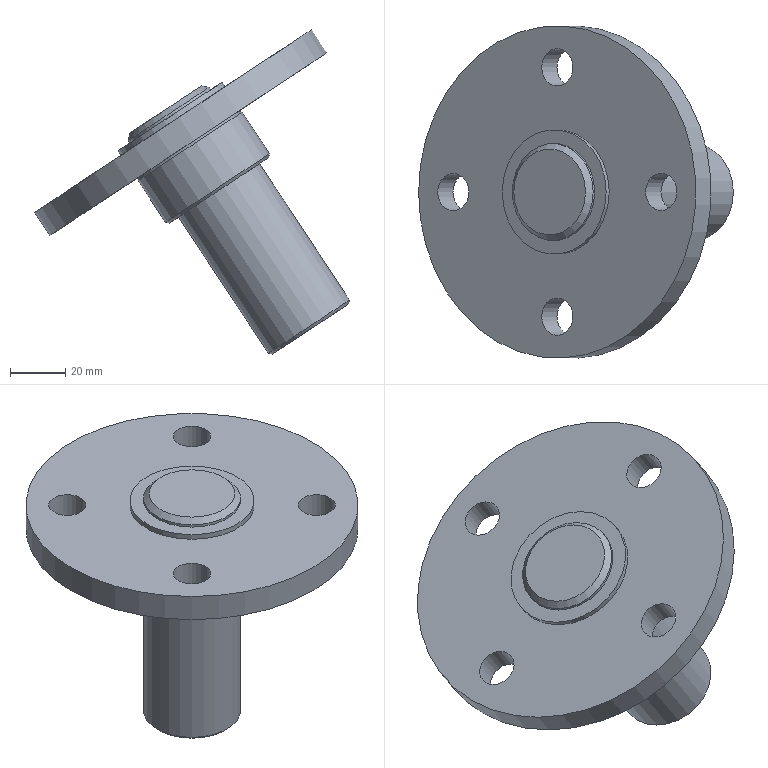Part | STEP file | HL4GZ-1.862.034 (flange rotating shaft) | 2 solids | 21 faces | box 113.701 x 120 x 117.252 mm | volume 202570 mm3 | cylinder 10 | plane 7 | cone 4 | commonest cylinder face diameters 13.5 x4 35 x3 45 x2 120 x1
STEP:
#1=CARTESIAN_POINT('',(0.,0.,0.));
#2=DIRECTION('',(0.,0.,1.));
#3=DIRECTION('',(1.,0.,0.));
#4=AXIS2_PLACEMENT_3D('',#1,#2,#3);
#5=CARTESIAN_POINT('',(3828.992,-590.,-108.754));
#6=VERTEX_POINT('',#5);
#7=CARTESIAN_POINT('',(3843.599,-590.,-99.117));
#8=DIRECTION('',(0.5507,0.,-0.8347));
#9=DIRECTION('',(-0.8347,0.,-0.5507));
#10=AXIS2_PLACEMENT_3D('',#7,#8,#9);
#11=CIRCLE('',#10,17.5);
#12=CARTESIAN_POINT('',(3843.599,-590.,-99.117));
#13=DIRECTION('',(0.5507,0.,-0.8347));
#14=DIRECTION('',(-0.8347,0.,-0.5507));
#15=AXIS2_PLACEMENT_3D('',#12,#13,#14);
#16=PLANE('',#15);
#17=CARTESIAN_POINT('',(0.,0.));
#18=DIRECTION('',(1.,0.));
#19=AXIS2_PLACEMENT_2D('',#17,#18);
#20=CIRCLE('',#19,17.5);
#21=(GEOMETRIC_REPRESENTATION_CONTEXT(2)PARAMETRIC_REPRESENTATION_CONTEXT()REPRESENTATION_CONTEXT('',''));
#22=DEFINITIONAL_REPRESENTATION('',(#20),#21);
#23=PCURVE('',#16,#22);
#24=CARTESIAN_POINT('',(3846.903,-590.,-104.125));
#25=DIRECTION('',(0.5507,0.,-0.8347));
#26=DIRECTION('',(0.8347,0.,0.5507));
#27=AXIS2_PLACEMENT_3D('',#24,#25,#26);
#28=CYLINDRICAL_SURFACE('',#27,17.5);
#29=CARTESIAN_POINT('',(3.142,-6.));
#30=DIRECTION('',(1.,0.));
#31=VECTOR('',#30,1.);
#32=LINE('',#29,#31);
#33=(GEOMETRIC_REPRESENTATION_CONTEXT(2)PARAMETRIC_REPRESENTATION_CONTEXT()REPRESENTATION_CONTEXT('',''));
#34=DEFINITIONAL_REPRESENTATION('',(#32),#33);
#35=PCURVE('',#28,#34);
#36=SURFACE_CURVE('',#11,(#23,#35),.PCURVE_S1.);
#37=EDGE_CURVE('',#6,#6,#36,.T.);
#38=ORIENTED_EDGE('',*,*,#37,.T.);
#39=EDGE_LOOP('',(#38));
#40=FACE_BOUND('',#39,.T.);
#41=CARTESIAN_POINT('',(3824.818,-590.,-111.507));
#42=VERTEX_POINT('',#41);
#43=CARTESIAN_POINT('',(3843.599,-590.,-99.117));
#44=DIRECTION('',(-0.5507,0.,0.8347));
#45=DIRECTION('',(-0.8347,0.,-0.5507));
#46=AXIS2_PLACEMENT_3D('',#43,#44,#45);
#47=CIRCLE('',#46,22.5);
#48=CARTESIAN_POINT('',(22.5,0.));
#49=CARTESIAN_POINT('',(22.5,-38.971));
#50=CARTESIAN_POINT('',(-11.25,-19.486));
#51=CARTESIAN_POINT('',(-45.,0.));
#52=CARTESIAN_POINT('',(-11.25,19.486));
#53=CARTESIAN_POINT('',(22.5,38.971));
#54=CARTESIAN_POINT('',(22.5,0.));
#55=(BOUNDED_CURVE()B_SPLINE_CURVE(2,(#48,#49,#50,#51,#52,#53,#54),.UNSPECIFIED.,.T.,.F.)B_SPLINE_CURVE_WITH_KNOTS((1,2,2,2,2,1),(-2.094,0.,2.094,4.189,6.283,8.378),.UNSPECIFIED.)CURVE()GEOMETRIC_REPRESENTATION_ITEM()RATIONAL_B_SPLINE_CURVE((1.,0.5,1.,0.5,1.,0.5,1.))REPRESENTATION_ITEM(''));
#56=(GEOMETRIC_REPRESENTATION_CONTEXT(2)PARAMETRIC_REPRESENTATION_CONTEXT()REPRESENTATION_CONTEXT('',''));
#57=DEFINITIONAL_REPRESENTATION('',(#55),#56);
#58=PCURVE('',#16,#57);
#59=CARTESIAN_POINT('',(3844.7,-590.,-100.786));
#60=DIRECTION('',(0.5507,0.,-0.8347));
#61=DIRECTION('',(0.8347,0.,0.5507));
#62=AXIS2_PLACEMENT_3D('',#59,#60,#61);
#63=CYLINDRICAL_SURFACE('',#62,22.5);
#64=CARTESIAN_POINT('',(9.425,-2.));
#65=DIRECTION('',(-1.,0.));
#66=VECTOR('',#65,1.);
#67=LINE('',#64,#66);
#68=(GEOMETRIC_REPRESENTATION_CONTEXT(2)PARAMETRIC_REPRESENTATION_CONTEXT()REPRESENTATION_CONTEXT('',''));
#69=DEFINITIONAL_REPRESENTATION('',(#67),#68);
#70=PCURVE('',#63,#69);
#71=SURFACE_CURVE('',#47,(#58,#70),.PCURVE_S1.);
#72=EDGE_CURVE('',#42,#42,#71,.T.);
#73=ORIENTED_EDGE('',*,*,#72,.T.);
#74=EDGE_LOOP('',(#73));
#75=FACE_BOUND('',#74,.T.);
#76=ADVANCED_FACE('',(#40,#75),#16,.F.);
#77=CARTESIAN_POINT('',(3825.919,-590.,-113.176));
#78=VERTEX_POINT('',#77);
#79=CARTESIAN_POINT('',(3844.7,-590.,-100.786));
#80=DIRECTION('',(-0.5507,0.,0.8347));
#81=DIRECTION('',(-0.8347,0.,-0.5507));
#82=AXIS2_PLACEMENT_3D('',#79,#80,#81);
#83=CIRCLE('',#82,22.5);
#84=CARTESIAN_POINT('',(9.425,0.));
#85=DIRECTION('',(-1.,0.));
#86=VECTOR('',#85,1.);
#87=LINE('',#84,#86);
#88=(GEOMETRIC_REPRESENTATION_CONTEXT(2)PARAMETRIC_REPRESENTATION_CONTEXT()REPRESENTATION_CONTEXT('',''));
#89=DEFINITIONAL_REPRESENTATION('',(#87),#88);
#90=PCURVE('',#63,#89);
#91=CARTESIAN_POINT('',(3844.7,-590.,-100.786));
#92=DIRECTION('',(0.5507,0.,-0.8347));
#93=DIRECTION('',(-0.8347,0.,-0.5507));
#94=AXIS2_PLACEMENT_3D('',#91,#92,#93);
#95=PLANE('',#94);
#96=CARTESIAN_POINT('',(22.5,0.));
#97=CARTESIAN_POINT('',(22.5,-38.971));
#98=CARTESIAN_POINT('',(-11.25,-19.486));
#99=CARTESIAN_POINT('',(-45.,0.));
#100=CARTESIAN_POINT('',(-11.25,19.486));
#101=CARTESIAN_POINT('',(22.5,38.971));
#102=CARTESIAN_POINT('',(22.5,0.));
#103=(BOUNDED_CURVE()B_SPLINE_CURVE(2,(#96,#97,#98,#99,#100,#101,#102),.UNSPECIFIED.,.T.,.F.)B_SPLINE_CURVE_WITH_KNOTS((1,2,2,2,2,1),(-2.094,0.,2.094,4.189,6.283,8.378),.UNSPECIFIED.)CURVE()GEOMETRIC_REPRESENTATION_ITEM()RATIONAL_B_SPLINE_CURVE((1.,0.5,1.,0.5,1.,0.5,1.))REPRESENTATION_ITEM(''));
#104=(GEOMETRIC_REPRESENTATION_CONTEXT(2)PARAMETRIC_REPRESENTATION_CONTEXT()REPRESENTATION_CONTEXT('',''));
#105=DEFINITIONAL_REPRESENTATION('',(#103),#104);
#106=PCURVE('',#95,#105);
#107=SURFACE_CURVE('',#83,(#90,#106),.PCURVE_S1.);
#108=EDGE_CURVE('',#78,#78,#107,.T.);
#109=ORIENTED_EDGE('',*,*,#108,.T.);
#110=CARTESIAN_POINT('',(3824.818,-590.,-111.507));
#111=CARTESIAN_POINT('',(3825.919,-590.,-113.176));
#112=B_SPLINE_CURVE_WITH_KNOTS('',1,(#110,#111),.UNSPECIFIED.,.F.,.F.,(2,2),(-2.,0.),.PIECEWISE_BEZIER_KNOTS.);
#113=CARTESIAN_POINT('',(3.142,0.));
#114=DIRECTION('',(0.,1.));
#115=VECTOR('',#114,1.);
#116=LINE('',#113,#115);
#117=(GEOMETRIC_REPRESENTATION_CONTEXT(2)PARAMETRIC_REPRESENTATION_CONTEXT()REPRESENTATION_CONTEXT('',''));
#118=DEFINITIONAL_REPRESENTATION('',(#116),#117);
#119=PCURVE('',#63,#118);
#120=CARTESIAN_POINT('',(9.425,0.));
#121=DIRECTION('',(0.,1.));
#122=VECTOR('',#121,1.);
#123=LINE('',#120,#122);
#124=(GEOMETRIC_REPRESENTATION_CONTEXT(2)PARAMETRIC_REPRESENTATION_CONTEXT()REPRESENTATION_CONTEXT('',''));
#125=DEFINITIONAL_REPRESENTATION('',(#123),#124);
#126=PCURVE('',#63,#125);
#127=SEAM_CURVE('',#112,(#119,#126),.PCURVE_S1.);
#128=EDGE_CURVE('',#42,#78,#127,.T.);
#129=ORIENTED_EDGE('',*,*,#128,.F.);
#130=ORIENTED_EDGE('',*,*,#72,.F.);
#131=ORIENTED_EDGE('',*,*,#128,.T.);
#132=EDGE_LOOP('',(#109,#129,#130,#131));
#133=FACE_BOUND('',#132,.T.);
#134=ADVANCED_FACE('',(#133),#63,.T.);
#135=CARTESIAN_POINT('',(3839.066,-545.,-104.503));
#136=VERTEX_POINT('',#135);
#137=CARTESIAN_POINT('',(3844.7,-545.,-100.786));
#138=DIRECTION('',(0.5507,0.,-0.8347));
#139=DIRECTION('',(-0.8347,0.,-0.5507));
#140=AXIS2_PLACEMENT_3D('',#137,#138,#139);
#141=CIRCLE('',#140,6.75);
#142=CARTESIAN_POINT('',(3839.193,-545.,-92.439));
#143=DIRECTION('',(0.5507,0.,-0.8347));
#144=DIRECTION('',(0.8347,0.,0.5507));
#145=AXIS2_PLACEMENT_3D('',#142,#143,#144);
#146=CYLINDRICAL_SURFACE('',#145,6.75);
#147=CARTESIAN_POINT('',(3.142,10.));
#148=DIRECTION('',(1.,0.));
#149=VECTOR('',#148,1.);
#150=LINE('',#147,#149);
#151=(GEOMETRIC_REPRESENTATION_CONTEXT(2)PARAMETRIC_REPRESENTATION_CONTEXT()REPRESENTATION_CONTEXT('',''));
#152=DEFINITIONAL_REPRESENTATION('',(#150),#151);
#153=PCURVE('',#146,#152);
#154=CARTESIAN_POINT('',(0.,45.));
#155=DIRECTION('',(1.,0.));
#156=AXIS2_PLACEMENT_2D('',#154,#155);
#157=CIRCLE('',#156,6.75);
#158=(GEOMETRIC_REPRESENTATION_CONTEXT(2)PARAMETRIC_REPRESENTATION_CONTEXT()REPRESENTATION_CONTEXT('',''));
#159=DEFINITIONAL_REPRESENTATION('',(#157),#158);
#160=PCURVE('',#95,#159);
#161=SURFACE_CURVE('',#141,(#153,#160),.PCURVE_S1.);
#162=EDGE_CURVE('',#136,#136,#161,.T.);
#163=ORIENTED_EDGE('',*,*,#162,.T.);
#164=CARTESIAN_POINT('',(3844.573,-545.,-112.85));
#165=VERTEX_POINT('',#164);
#166=CARTESIAN_POINT('',(3839.066,-545.,-104.503));
#167=CARTESIAN_POINT('',(3844.573,-545.,-112.85));
#168=B_SPLINE_CURVE_WITH_KNOTS('',1,(#166,#167),.UNSPECIFIED.,.F.,.F.,(2,2),(10.,20.),.PIECEWISE_BEZIER_KNOTS.);
#169=CARTESIAN_POINT('',(9.425,0.));
#170=DIRECTION('',(0.,1.));
#171=VECTOR('',#170,1.);
#172=LINE('',#169,#171);
#173=(GEOMETRIC_REPRESENTATION_CONTEXT(2)PARAMETRIC_REPRESENTATION_CONTEXT()REPRESENTATION_CONTEXT('',''));
#174=DEFINITIONAL_REPRESENTATION('',(#172),#173);
#175=PCURVE('',#146,#174);
#176=CARTESIAN_POINT('',(3.142,0.));
#177=DIRECTION('',(0.,1.));
#178=VECTOR('',#177,1.);
#179=LINE('',#176,#178);
#180=(GEOMETRIC_REPRESENTATION_CONTEXT(2)PARAMETRIC_REPRESENTATION_CONTEXT()REPRESENTATION_CONTEXT('',''));
#181=DEFINITIONAL_REPRESENTATION('',(#179),#180);
#182=PCURVE('',#146,#181);
#183=SEAM_CURVE('',#168,(#175,#182),.PCURVE_S1.);
#184=EDGE_CURVE('',#136,#165,#183,.T.);
#185=ORIENTED_EDGE('',*,*,#184,.T.);
#186=CARTESIAN_POINT('',(3850.207,-545.,-109.133));
#187=DIRECTION('',(0.5507,0.,-0.8347));
#188=DIRECTION('',(-0.8347,0.,-0.5507));
#189=AXIS2_PLACEMENT_3D('',#186,#187,#188);
#190=CIRCLE('',#189,6.75);
#191=CARTESIAN_POINT('',(3.142,20.));
#192=DIRECTION('',(1.,0.));
#193=VECTOR('',#192,1.);
#194=LINE('',#191,#193);
#195=(GEOMETRIC_REPRESENTATION_CONTEXT(2)PARAMETRIC_REPRESENTATION_CONTEXT()REPRESENTATION_CONTEXT('',''));
#196=DEFINITIONAL_REPRESENTATION('',(#194),#195);
#197=PCURVE('',#146,#196);
#198=CARTESIAN_POINT('',(3850.207,-590.,-109.133));
#199=DIRECTION('',(0.5507,0.,-0.8347));
#200=DIRECTION('',(-0.8347,0.,-0.5507));
#201=AXIS2_PLACEMENT_3D('',#198,#199,#200);
#202=PLANE('',#201);
#203=CARTESIAN_POINT('',(0.,45.));
#204=DIRECTION('',(1.,0.));
#205=AXIS2_PLACEMENT_2D('',#203,#204);
#206=CIRCLE('',#205,6.75);
#207=(GEOMETRIC_REPRESENTATION_CONTEXT(2)PARAMETRIC_REPRESENTATION_CONTEXT()REPRESENTATION_CONTEXT('',''));
#208=DEFINITIONAL_REPRESENTATION('',(#206),#207);
#209=PCURVE('',#202,#208);
#210=SURFACE_CURVE('',#190,(#197,#209),.PCURVE_S1.);
#211=EDGE_CURVE('',#165,#165,#210,.T.);
#212=ORIENTED_EDGE('',*,*,#211,.F.);
#213=ORIENTED_EDGE('',*,*,#184,.F.);
#214=EDGE_LOOP('',(#163,#185,#212,#213));
#215=FACE_BOUND('',#214,.F.);
#216=ADVANCED_FACE('',(#215),#146,.F.);
#217=CARTESIAN_POINT('',(3801.504,-590.,-129.284));
#218=VERTEX_POINT('',#217);
#219=CARTESIAN_POINT('',(3807.138,-590.,-125.567));
#220=DIRECTION('',(0.5507,0.,-0.8347));
#221=DIRECTION('',(-0.8347,0.,-0.5507));
#222=AXIS2_PLACEMENT_3D('',#219,#220,#221);
#223=CIRCLE('',#222,6.75);
#224=CARTESIAN_POINT('',(3801.631,-590.,-117.22));
#225=DIRECTION('',(0.5507,0.,-0.8347));
#226=DIRECTION('',(0.8347,0.,0.5507));
#227=AXIS2_PLACEMENT_3D('',#224,#225,#226);
#228=CYLINDRICAL_SURFACE('',#227,6.75);
#229=CARTESIAN_POINT('',(3.142,10.));
#230=DIRECTION('',(1.,0.));
#231=VECTOR('',#230,1.);
#232=LINE('',#229,#231);
#233=(GEOMETRIC_REPRESENTATION_CONTEXT(2)PARAMETRIC_REPRESENTATION_CONTEXT()REPRESENTATION_CONTEXT('',''));
#234=DEFINITIONAL_REPRESENTATION('',(#232),#233);
#235=PCURVE('',#228,#234);
#236=CARTESIAN_POINT('',(45.,0.));
#237=DIRECTION('',(1.,0.));
#238=AXIS2_PLACEMENT_2D('',#236,#237);
#239=CIRCLE('',#238,6.75);
#240=(GEOMETRIC_REPRESENTATION_CONTEXT(2)PARAMETRIC_REPRESENTATION_CONTEXT()REPRESENTATION_CONTEXT('',''));
#241=DEFINITIONAL_REPRESENTATION('',(#239),#240);
#242=PCURVE('',#95,#241);
#243=SURFACE_CURVE('',#223,(#235,#242),.PCURVE_S1.);
#244=EDGE_CURVE('',#218,#218,#243,.T.);
#245=ORIENTED_EDGE('',*,*,#244,.T.);
#246=CARTESIAN_POINT('',(3807.011,-590.,-137.631));
#247=VERTEX_POINT('',#246);
#248=CARTESIAN_POINT('',(3801.504,-590.,-129.284));
#249=CARTESIAN_POINT('',(3807.011,-590.,-137.631));
#250=B_SPLINE_CURVE_WITH_KNOTS('',1,(#248,#249),.UNSPECIFIED.,.F.,.F.,(2,2),(10.,20.),.PIECEWISE_BEZIER_KNOTS.);
#251=CARTESIAN_POINT('',(9.425,0.));
#252=DIRECTION('',(0.,1.));
#253=VECTOR('',#252,1.);
#254=LINE('',#251,#253);
#255=(GEOMETRIC_REPRESENTATION_CONTEXT(2)PARAMETRIC_REPRESENTATION_CONTEXT()REPRESENTATION_CONTEXT('',''));
#256=DEFINITIONAL_REPRESENTATION('',(#254),#255);
#257=PCURVE('',#228,#256);
#258=CARTESIAN_POINT('',(3.142,0.));
#259=DIRECTION('',(0.,1.));
#260=VECTOR('',#259,1.);
#261=LINE('',#258,#260);
#262=(GEOMETRIC_REPRESENTATION_CONTEXT(2)PARAMETRIC_REPRESENTATION_CONTEXT()REPRESENTATION_CONTEXT('',''));
#263=DEFINITIONAL_REPRESENTATION('',(#261),#262);
#264=PCURVE('',#228,#263);
#265=SEAM_CURVE('',#250,(#257,#264),.PCURVE_S1.);
#266=EDGE_CURVE('',#218,#247,#265,.T.);
#267=ORIENTED_EDGE('',*,*,#266,.T.);
#268=CARTESIAN_POINT('',(3812.645,-590.,-133.914));
#269=DIRECTION('',(0.5507,0.,-0.8347));
#270=DIRECTION('',(-0.8347,0.,-0.5507));
#271=AXIS2_PLACEMENT_3D('',#268,#269,#270);
#272=CIRCLE('',#271,6.75);
#273=CARTESIAN_POINT('',(3.142,20.));
#274=DIRECTION('',(1.,0.));
#275=VECTOR('',#274,1.);
#276=LINE('',#273,#275);
#277=(GEOMETRIC_REPRESENTATION_CONTEXT(2)PARAMETRIC_REPRESENTATION_CONTEXT()REPRESENTATION_CONTEXT('',''));
#278=DEFINITIONAL_REPRESENTATION('',(#276),#277);
#279=PCURVE('',#228,#278);
#280=CARTESIAN_POINT('',(45.,0.));
#281=DIRECTION('',(1.,0.));
#282=AXIS2_PLACEMENT_2D('',#280,#281);
#283=CIRCLE('',#282,6.75);
#284=(GEOMETRIC_REPRESENTATION_CONTEXT(2)PARAMETRIC_REPRESENTATION_CONTEXT()REPRESENTATION_CONTEXT('',''));
#285=DEFINITIONAL_REPRESENTATION('',(#283),#284);
#286=PCURVE('',#202,#285);
#287=SURFACE_CURVE('',#272,(#279,#286),.PCURVE_S1.);
#288=EDGE_CURVE('',#247,#247,#287,.T.);
#289=ORIENTED_EDGE('',*,*,#288,.F.);
#290=ORIENTED_EDGE('',*,*,#266,.F.);
#291=EDGE_LOOP('',(#245,#267,#289,#290));
#292=FACE_BOUND('',#291,.F.);
#293=ADVANCED_FACE('',(#292),#228,.F.);
#294=CARTESIAN_POINT('',(3839.066,-635.,-104.503));
#295=VERTEX_POINT('',#294);
#296=CARTESIAN_POINT('',(3844.7,-635.,-100.786));
#297=DIRECTION('',(0.5507,0.,-0.8347));
#298=DIRECTION('',(-0.8347,0.,-0.5507));
#299=AXIS2_PLACEMENT_3D('',#296,#297,#298);
#300=CIRCLE('',#299,6.75);
#301=CARTESIAN_POINT('',(3839.193,-635.,-92.439));
#302=DIRECTION('',(0.5507,0.,-0.8347));
#303=DIRECTION('',(0.8347,0.,0.5507));
#304=AXIS2_PLACEMENT_3D('',#301,#302,#303);
#305=CYLINDRICAL_SURFACE('',#304,6.75);
#306=CARTESIAN_POINT('',(3.142,10.));
#307=DIRECTION('',(1.,0.));
#308=VECTOR('',#307,1.);
#309=LINE('',#306,#308);
#310=(GEOMETRIC_REPRESENTATION_CONTEXT(2)PARAMETRIC_REPRESENTATION_CONTEXT()REPRESENTATION_CONTEXT('',''));
#311=DEFINITIONAL_REPRESENTATION('',(#309),#310);
#312=PCURVE('',#305,#311);
#313=CARTESIAN_POINT('',(0.,-45.));
#314=DIRECTION('',(1.,0.));
#315=AXIS2_PLACEMENT_2D('',#313,#314);
#316=CIRCLE('',#315,6.75);
#317=(GEOMETRIC_REPRESENTATION_CONTEXT(2)PARAMETRIC_REPRESENTATION_CONTEXT()REPRESENTATION_CONTEXT('',''));
#318=DEFINITIONAL_REPRESENTATION('',(#316),#317);
#319=PCURVE('',#95,#318);
#320=SURFACE_CURVE('',#300,(#312,#319),.PCURVE_S1.);
#321=EDGE_CURVE('',#295,#295,#320,.T.);
#322=ORIENTED_EDGE('',*,*,#321,.T.);
#323=CARTESIAN_POINT('',(3844.573,-635.,-112.85));
#324=VERTEX_POINT('',#323);
#325=CARTESIAN_POINT('',(3839.066,-635.,-104.503));
#326=CARTESIAN_POINT('',(3844.573,-635.,-112.85));
#327=B_SPLINE_CURVE_WITH_KNOTS('',1,(#325,#326),.UNSPECIFIED.,.F.,.F.,(2,2),(10.,20.),.PIECEWISE_BEZIER_KNOTS.);
#328=CARTESIAN_POINT('',(9.425,0.));
#329=DIRECTION('',(0.,1.));
#330=VECTOR('',#329,1.);
#331=LINE('',#328,#330);
#332=(GEOMETRIC_REPRESENTATION_CONTEXT(2)PARAMETRIC_REPRESENTATION_CONTEXT()REPRESENTATION_CONTEXT('',''));
#333=DEFINITIONAL_REPRESENTATION('',(#331),#332);
#334=PCURVE('',#305,#333);
#335=CARTESIAN_POINT('',(3.142,0.));
#336=DIRECTION('',(0.,1.));
#337=VECTOR('',#336,1.);
#338=LINE('',#335,#337);
#339=(GEOMETRIC_REPRESENTATION_CONTEXT(2)PARAMETRIC_REPRESENTATION_CONTEXT()REPRESENTATION_CONTEXT('',''));
#340=DEFINITIONAL_REPRESENTATION('',(#338),#339);
#341=PCURVE('',#305,#340);
#342=SEAM_CURVE('',#327,(#334,#341),.PCURVE_S1.);
#343=EDGE_CURVE('',#295,#324,#342,.T.);
#344=ORIENTED_EDGE('',*,*,#343,.T.);
#345=CARTESIAN_POINT('',(3850.207,-635.,-109.133));
#346=DIRECTION('',(0.5507,0.,-0.8347));
#347=DIRECTION('',(-0.8347,0.,-0.5507));
#348=AXIS2_PLACEMENT_3D('',#345,#346,#347);
#349=CIRCLE('',#348,6.75);
#350=CARTESIAN_POINT('',(3.142,20.));
#351=DIRECTION('',(1.,0.));
#352=VECTOR('',#351,1.);
#353=LINE('',#350,#352);
#354=(GEOMETRIC_REPRESENTATION_CONTEXT(2)PARAMETRIC_REPRESENTATION_CONTEXT()REPRESENTATION_CONTEXT('',''));
#355=DEFINITIONAL_REPRESENTATION('',(#353),#354);
#356=PCURVE('',#305,#355);
#357=CARTESIAN_POINT('',(0.,-45.));
#358=DIRECTION('',(1.,0.));
#359=AXIS2_PLACEMENT_2D('',#357,#358);
#360=CIRCLE('',#359,6.75);
#361=(GEOMETRIC_REPRESENTATION_CONTEXT(2)PARAMETRIC_REPRESENTATION_CONTEXT()REPRESENTATION_CONTEXT('',''));
#362=DEFINITIONAL_REPRESENTATION('',(#360),#361);
#363=PCURVE('',#202,#362);
#364=SURFACE_CURVE('',#349,(#356,#363),.PCURVE_S1.);
#365=EDGE_CURVE('',#324,#324,#364,.T.);
#366=ORIENTED_EDGE('',*,*,#365,.F.);
#367=ORIENTED_EDGE('',*,*,#343,.F.);
#368=EDGE_LOOP('',(#322,#344,#366,#367));
#369=FACE_BOUND('',#368,.F.);
#370=ADVANCED_FACE('',(#369),#305,.F.);
#371=CARTESIAN_POINT('',(3876.628,-590.,-79.722));
#372=VERTEX_POINT('',#371);
#373=CARTESIAN_POINT('',(3882.262,-590.,-76.005));
#374=DIRECTION('',(-0.5507,0.,0.8347));
#375=DIRECTION('',(-0.8347,0.,-0.5507));
#376=AXIS2_PLACEMENT_3D('',#373,#374,#375);
#377=CIRCLE('',#376,6.75);
#378=CARTESIAN_POINT('',(3876.756,-590.,-67.658));
#379=DIRECTION('',(0.5507,0.,-0.8347));
#380=DIRECTION('',(0.8347,0.,0.5507));
#381=AXIS2_PLACEMENT_3D('',#378,#379,#380);
#382=CYLINDRICAL_SURFACE('',#381,6.75);
#383=CARTESIAN_POINT('',(9.425,10.));
#384=DIRECTION('',(-1.,0.));
#385=VECTOR('',#384,1.);
#386=LINE('',#383,#385);
#387=(GEOMETRIC_REPRESENTATION_CONTEXT(2)PARAMETRIC_REPRESENTATION_CONTEXT()REPRESENTATION_CONTEXT('',''));
#388=DEFINITIONAL_REPRESENTATION('',(#386),#387);
#389=PCURVE('',#382,#388);
#390=CARTESIAN_POINT('',(-38.25,0.));
#391=CARTESIAN_POINT('',(-38.25,-11.691));
#392=CARTESIAN_POINT('',(-48.375,-5.846));
#393=CARTESIAN_POINT('',(-58.5,0.));
#394=CARTESIAN_POINT('',(-48.375,5.846));
#395=CARTESIAN_POINT('',(-38.25,11.691));
#396=CARTESIAN_POINT('',(-38.25,0.));
#397=(BOUNDED_CURVE()B_SPLINE_CURVE(2,(#390,#391,#392,#393,#394,#395,#396),.UNSPECIFIED.,.T.,.F.)B_SPLINE_CURVE_WITH_KNOTS((1,2,2,2,2,1),(-2.094,0.,2.094,4.189,6.283,8.378),.UNSPECIFIED.)CURVE()GEOMETRIC_REPRESENTATION_ITEM()RATIONAL_B_SPLINE_CURVE((1.,0.5,1.,0.5,1.,0.5,1.))REPRESENTATION_ITEM(''));
#398=(GEOMETRIC_REPRESENTATION_CONTEXT(2)PARAMETRIC_REPRESENTATION_CONTEXT()REPRESENTATION_CONTEXT('',''));
#399=DEFINITIONAL_REPRESENTATION('',(#397),#398);
#400=PCURVE('',#95,#399);
#401=SURFACE_CURVE('',#377,(#389,#400),.PCURVE_S1.);
#402=EDGE_CURVE('',#372,#372,#401,.T.);
#403=ORIENTED_EDGE('',*,*,#402,.F.);
#404=CARTESIAN_POINT('',(3882.135,-590.,-88.069));
#405=VERTEX_POINT('',#404);
#406=CARTESIAN_POINT('',(3876.628,-590.,-79.722));
#407=CARTESIAN_POINT('',(3882.135,-590.,-88.069));
#408=B_SPLINE_CURVE_WITH_KNOTS('',1,(#406,#407),.UNSPECIFIED.,.F.,.F.,(2,2),(10.,20.),.PIECEWISE_BEZIER_KNOTS.);
#409=CARTESIAN_POINT('',(9.425,0.));
#410=DIRECTION('',(0.,1.));
#411=VECTOR('',#410,1.);
#412=LINE('',#409,#411);
#413=(GEOMETRIC_REPRESENTATION_CONTEXT(2)PARAMETRIC_REPRESENTATION_CONTEXT()REPRESENTATION_CONTEXT('',''));
#414=DEFINITIONAL_REPRESENTATION('',(#412),#413);
#415=PCURVE('',#382,#414);
#416=CARTESIAN_POINT('',(3.142,0.));
#417=DIRECTION('',(0.,1.));
#418=VECTOR('',#417,1.);
#419=LINE('',#416,#418);
#420=(GEOMETRIC_REPRESENTATION_CONTEXT(2)PARAMETRIC_REPRESENTATION_CONTEXT()REPRESENTATION_CONTEXT('',''));
#421=DEFINITIONAL_REPRESENTATION('',(#419),#420);
#422=PCURVE('',#382,#421);
#423=SEAM_CURVE('',#408,(#415,#422),.PCURVE_S1.);
#424=EDGE_CURVE('',#372,#405,#423,.T.);
#425=ORIENTED_EDGE('',*,*,#424,.T.);
#426=CARTESIAN_POINT('',(3887.769,-590.,-84.352));
#427=DIRECTION('',(-0.5507,0.,0.8347));
#428=DIRECTION('',(-0.8347,0.,-0.5507));
#429=AXIS2_PLACEMENT_3D('',#426,#427,#428);
#430=CIRCLE('',#429,6.75);
#431=CARTESIAN_POINT('',(9.425,20.));
#432=DIRECTION('',(-1.,0.));
#433=VECTOR('',#432,1.);
#434=LINE('',#431,#433);
#435=(GEOMETRIC_REPRESENTATION_CONTEXT(2)PARAMETRIC_REPRESENTATION_CONTEXT()REPRESENTATION_CONTEXT('',''));
#436=DEFINITIONAL_REPRESENTATION('',(#434),#435);
#437=PCURVE('',#382,#436);
#438=CARTESIAN_POINT('',(-38.25,0.));
#439=CARTESIAN_POINT('',(-38.25,-11.691));
#440=CARTESIAN_POINT('',(-48.375,-5.846));
#441=CARTESIAN_POINT('',(-58.5,0.));
#442=CARTESIAN_POINT('',(-48.375,5.846));
#443=CARTESIAN_POINT('',(-38.25,11.691));
#444=CARTESIAN_POINT('',(-38.25,0.));
#445=(BOUNDED_CURVE()B_SPLINE_CURVE(2,(#438,#439,#440,#441,#442,#443,#444),.UNSPECIFIED.,.T.,.F.)B_SPLINE_CURVE_WITH_KNOTS((1,2,2,2,2,1),(-2.094,0.,2.094,4.189,6.283,8.378),.UNSPECIFIED.)CURVE()GEOMETRIC_REPRESENTATION_ITEM()RATIONAL_B_SPLINE_CURVE((1.,0.5,1.,0.5,1.,0.5,1.))REPRESENTATION_ITEM(''));
#446=(GEOMETRIC_REPRESENTATION_CONTEXT(2)PARAMETRIC_REPRESENTATION_CONTEXT()REPRESENTATION_CONTEXT('',''));
#447=DEFINITIONAL_REPRESENTATION('',(#445),#446);
#448=PCURVE('',#202,#447);
#449=SURFACE_CURVE('',#430,(#437,#448),.PCURVE_S1.);
#450=EDGE_CURVE('',#405,#405,#449,.T.);
#451=ORIENTED_EDGE('',*,*,#450,.T.);
#452=ORIENTED_EDGE('',*,*,#424,.F.);
#453=EDGE_LOOP('',(#403,#425,#451,#452));
#454=FACE_BOUND('',#453,.F.);
#455=ADVANCED_FACE('',(#454),#382,.F.);
#456=CARTESIAN_POINT('',(3835.6,-590.,-118.77));
#457=VERTEX_POINT('',#456);
#458=CARTESIAN_POINT('',(3850.207,-590.,-109.133));
#459=DIRECTION('',(-0.5507,0.,0.8347));
#460=DIRECTION('',(0.8347,0.,0.5507));
#461=AXIS2_PLACEMENT_3D('',#458,#459,#460);
#462=CIRCLE('',#461,17.5);
#463=CARTESIAN_POINT('',(-17.5,0.));
#464=CARTESIAN_POINT('',(-17.5,30.311));
#465=CARTESIAN_POINT('',(8.75,15.155));
#466=CARTESIAN_POINT('',(35.,0.));
#467=CARTESIAN_POINT('',(8.75,-15.155));
#468=CARTESIAN_POINT('',(-17.5,-30.311));
#469=CARTESIAN_POINT('',(-17.5,0.));
#470=(BOUNDED_CURVE()B_SPLINE_CURVE(2,(#463,#464,#465,#466,#467,#468,#469),.UNSPECIFIED.,.T.,.F.)B_SPLINE_CURVE_WITH_KNOTS((1,2,2,2,2,1),(-2.094,0.,2.094,4.189,6.283,8.378),.UNSPECIFIED.)CURVE()GEOMETRIC_REPRESENTATION_ITEM()RATIONAL_B_SPLINE_CURVE((1.,0.5,1.,0.5,1.,0.5,1.))REPRESENTATION_ITEM(''));
#471=(GEOMETRIC_REPRESENTATION_CONTEXT(2)PARAMETRIC_REPRESENTATION_CONTEXT()REPRESENTATION_CONTEXT('',''));
#472=DEFINITIONAL_REPRESENTATION('',(#470),#471);
#473=PCURVE('',#202,#472);
#474=CARTESIAN_POINT('',(12.566,6.));
#475=DIRECTION('',(-1.,0.));
#476=VECTOR('',#475,1.);
#477=LINE('',#474,#476);
#478=(GEOMETRIC_REPRESENTATION_CONTEXT(2)PARAMETRIC_REPRESENTATION_CONTEXT()REPRESENTATION_CONTEXT('',''));
#479=DEFINITIONAL_REPRESENTATION('',(#477),#478);
#480=PCURVE('',#28,#479);
#481=SURFACE_CURVE('',#462,(#473,#480),.PCURVE_S1.);
#482=EDGE_CURVE('',#457,#457,#481,.T.);
#483=ORIENTED_EDGE('',*,*,#482,.T.);
#484=EDGE_LOOP('',(#483));
#485=FACE_BOUND('',#484,.T.);
#486=CARTESIAN_POINT('',(3800.124,-590.,-142.174));
#487=VERTEX_POINT('',#486);
#488=CARTESIAN_POINT('',(3850.207,-590.,-109.133));
#489=DIRECTION('',(0.5507,0.,-0.8347));
#490=DIRECTION('',(-0.8347,0.,-0.5507));
#491=AXIS2_PLACEMENT_3D('',#488,#489,#490);
#492=CIRCLE('',#491,60.);
#493=CARTESIAN_POINT('',(0.,0.));
#494=DIRECTION('',(1.,0.));
#495=AXIS2_PLACEMENT_2D('',#493,#494);
#496=CIRCLE('',#495,60.);
#497=(GEOMETRIC_REPRESENTATION_CONTEXT(2)PARAMETRIC_REPRESENTATION_CONTEXT()REPRESENTATION_CONTEXT('',''));
#498=DEFINITIONAL_REPRESENTATION('',(#496),#497);
#499=PCURVE('',#202,#498);
#500=CARTESIAN_POINT('',(3846.903,-590.,-104.125));
#501=DIRECTION('',(0.5507,0.,-0.8347));
#502=DIRECTION('',(0.8347,0.,0.5507));
#503=AXIS2_PLACEMENT_3D('',#500,#501,#502);
#504=CYLINDRICAL_SURFACE('',#503,60.);
#505=CARTESIAN_POINT('',(3.142,6.));
#506=DIRECTION('',(1.,0.));
#507=VECTOR('',#506,1.);
#508=LINE('',#505,#507);
#509=(GEOMETRIC_REPRESENTATION_CONTEXT(2)PARAMETRIC_REPRESENTATION_CONTEXT()REPRESENTATION_CONTEXT('',''));
#510=DEFINITIONAL_REPRESENTATION('',(#508),#509);
#511=PCURVE('',#504,#510);
#512=SURFACE_CURVE('',#492,(#499,#511),.PCURVE_S1.);
#513=EDGE_CURVE('',#487,#487,#512,.T.);
#514=ORIENTED_EDGE('',*,*,#513,.T.);
#515=EDGE_LOOP('',(#514));
#516=FACE_BOUND('',#515,.T.);
#517=ORIENTED_EDGE('',*,*,#450,.T.);
#518=EDGE_LOOP('',(#517));
#519=FACE_BOUND('',#518,.T.);
#520=ORIENTED_EDGE('',*,*,#365,.F.);
#521=EDGE_LOOP('',(#520));
#522=FACE_BOUND('',#521,.T.);
#523=ORIENTED_EDGE('',*,*,#288,.F.);
#524=EDGE_LOOP('',(#523));
#525=FACE_BOUND('',#524,.T.);
#526=ORIENTED_EDGE('',*,*,#211,.F.);
#527=EDGE_LOOP('',(#526));
#528=FACE_BOUND('',#527,.T.);
#529=ADVANCED_FACE('',(#485,#516,#519,#522,#525,#528),#202,.T.);
#530=CARTESIAN_POINT('',(3794.618,-590.,-133.827));
#531=VERTEX_POINT('',#530);
#532=CARTESIAN_POINT('',(3844.7,-590.,-100.786));
#533=DIRECTION('',(-0.5507,0.,0.8347));
#534=DIRECTION('',(-0.8347,0.,-0.5507));
#535=AXIS2_PLACEMENT_3D('',#532,#533,#534);
#536=CIRCLE('',#535,60.);
#537=CARTESIAN_POINT('',(9.425,-4.));
#538=DIRECTION('',(-1.,0.));
#539=VECTOR('',#538,1.);
#540=LINE('',#537,#539);
#541=(GEOMETRIC_REPRESENTATION_CONTEXT(2)PARAMETRIC_REPRESENTATION_CONTEXT()REPRESENTATION_CONTEXT('',''));
#542=DEFINITIONAL_REPRESENTATION('',(#540),#541);
#543=PCURVE('',#504,#542);
#544=CARTESIAN_POINT('',(60.,0.));
#545=CARTESIAN_POINT('',(60.,-103.923));
#546=CARTESIAN_POINT('',(-30.,-51.962));
#547=CARTESIAN_POINT('',(-120.,0.));
#548=CARTESIAN_POINT('',(-30.,51.962));
#549=CARTESIAN_POINT('',(60.,103.923));
#550=CARTESIAN_POINT('',(60.,0.));
#551=(BOUNDED_CURVE()B_SPLINE_CURVE(2,(#544,#545,#546,#547,#548,#549,#550),.UNSPECIFIED.,.T.,.F.)B_SPLINE_CURVE_WITH_KNOTS((1,2,2,2,2,1),(-2.094,0.,2.094,4.189,6.283,8.378),.UNSPECIFIED.)CURVE()GEOMETRIC_REPRESENTATION_ITEM()RATIONAL_B_SPLINE_CURVE((1.,0.5,1.,0.5,1.,0.5,1.))REPRESENTATION_ITEM(''));
#552=(GEOMETRIC_REPRESENTATION_CONTEXT(2)PARAMETRIC_REPRESENTATION_CONTEXT()REPRESENTATION_CONTEXT('',''));
#553=DEFINITIONAL_REPRESENTATION('',(#551),#552);
#554=PCURVE('',#95,#553);
#555=SURFACE_CURVE('',#536,(#543,#554),.PCURVE_S1.);
#556=EDGE_CURVE('',#531,#531,#555,.T.);
#557=ORIENTED_EDGE('',*,*,#556,.F.);
#558=CARTESIAN_POINT('',(3794.618,-590.,-133.827));
#559=CARTESIAN_POINT('',(3800.124,-590.,-142.174));
#560=B_SPLINE_CURVE_WITH_KNOTS('',1,(#558,#559),.UNSPECIFIED.,.F.,.F.,(2,2),(-4.,6.),.PIECEWISE_BEZIER_KNOTS.);
#561=CARTESIAN_POINT('',(9.425,0.));
#562=DIRECTION('',(0.,1.));
#563=VECTOR('',#562,1.);
#564=LINE('',#561,#563);
#565=(GEOMETRIC_REPRESENTATION_CONTEXT(2)PARAMETRIC_REPRESENTATION_CONTEXT()REPRESENTATION_CONTEXT('',''));
#566=DEFINITIONAL_REPRESENTATION('',(#564),#565);
#567=PCURVE('',#504,#566);
#568=CARTESIAN_POINT('',(3.142,0.));
#569=DIRECTION('',(0.,1.));
#570=VECTOR('',#569,1.);
#571=LINE('',#568,#570);
#572=(GEOMETRIC_REPRESENTATION_CONTEXT(2)PARAMETRIC_REPRESENTATION_CONTEXT()REPRESENTATION_CONTEXT('',''));
#573=DEFINITIONAL_REPRESENTATION('',(#571),#572);
#574=PCURVE('',#504,#573);
#575=SEAM_CURVE('',#560,(#567,#574),.PCURVE_S1.);
#576=EDGE_CURVE('',#531,#487,#575,.T.);
#577=ORIENTED_EDGE('',*,*,#576,.T.);
#578=ORIENTED_EDGE('',*,*,#513,.F.);
#579=ORIENTED_EDGE('',*,*,#576,.F.);
#580=EDGE_LOOP('',(#557,#577,#578,#579));
#581=FACE_BOUND('',#580,.T.);
#582=ADVANCED_FACE('',(#581),#504,.T.);
#583=ORIENTED_EDGE('',*,*,#37,.T.);
#584=CARTESIAN_POINT('',(3828.992,-590.,-108.754));
#585=CARTESIAN_POINT('',(3835.6,-590.,-118.77));
#586=B_SPLINE_CURVE_WITH_KNOTS('',1,(#584,#585),.UNSPECIFIED.,.F.,.F.,(2,2),(-6.,6.),.PIECEWISE_BEZIER_KNOTS.);
#587=CARTESIAN_POINT('',(9.425,0.));
#588=DIRECTION('',(0.,1.));
#589=VECTOR('',#588,1.);
#590=LINE('',#587,#589);
#591=(GEOMETRIC_REPRESENTATION_CONTEXT(2)PARAMETRIC_REPRESENTATION_CONTEXT()REPRESENTATION_CONTEXT('',''));
#592=DEFINITIONAL_REPRESENTATION('',(#590),#591);
#593=PCURVE('',#28,#592);
#594=CARTESIAN_POINT('',(3.142,0.));
#595=DIRECTION('',(0.,1.));
#596=VECTOR('',#595,1.);
#597=LINE('',#594,#596);
#598=(GEOMETRIC_REPRESENTATION_CONTEXT(2)PARAMETRIC_REPRESENTATION_CONTEXT()REPRESENTATION_CONTEXT('',''));
#599=DEFINITIONAL_REPRESENTATION('',(#597),#598);
#600=PCURVE('',#28,#599);
#601=SEAM_CURVE('',#586,(#593,#600),.PCURVE_S1.);
#602=EDGE_CURVE('',#6,#457,#601,.T.);
#603=ORIENTED_EDGE('',*,*,#602,.T.);
#604=ORIENTED_EDGE('',*,*,#482,.T.);
#605=ORIENTED_EDGE('',*,*,#602,.F.);
#606=EDGE_LOOP('',(#583,#603,#604,#605));
#607=FACE_BOUND('',#606,.F.);
#608=ADVANCED_FACE('',(#607),#28,.F.);
#609=ORIENTED_EDGE('',*,*,#108,.F.);
#610=EDGE_LOOP('',(#609));
#611=FACE_BOUND('',#610,.T.);
#612=ORIENTED_EDGE('',*,*,#162,.T.);
#613=EDGE_LOOP('',(#612));
#614=FACE_BOUND('',#613,.T.);
#615=ORIENTED_EDGE('',*,*,#244,.T.);
#616=EDGE_LOOP('',(#615));
#617=FACE_BOUND('',#616,.T.);
#618=ORIENTED_EDGE('',*,*,#321,.T.);
#619=EDGE_LOOP('',(#618));
#620=FACE_BOUND('',#619,.T.);
#621=ORIENTED_EDGE('',*,*,#402,.F.);
#622=EDGE_LOOP('',(#621));
#623=FACE_BOUND('',#622,.T.);
#624=ORIENTED_EDGE('',*,*,#556,.T.);
#625=EDGE_LOOP('',(#624));
#626=FACE_BOUND('',#625,.T.);
#627=ADVANCED_FACE('',(#611,#614,#617,#620,#623,#626),#95,.F.);
#628=CLOSED_SHELL('',(#76,#134,#216,#293,#370,#455,#529,#582,#608,#627));
#629=MANIFOLD_SOLID_BREP('',#628);
#630=CARTESIAN_POINT('',(3908.319,-590.,-165.438));
#631=VERTEX_POINT('',#630);
#632=CARTESIAN_POINT('',(3879.104,-590.,-184.712));
#633=VERTEX_POINT('',#632);
#634=CARTESIAN_POINT('',(3893.711,-590.,-175.075));
#635=DIRECTION('',(0.5507,0.,-0.8347));
#636=DIRECTION('',(0.8347,0.,0.5507));
#637=AXIS2_PLACEMENT_3D('',#634,#635,#636);
#638=CIRCLE('',#637,17.5);
#639=CARTESIAN_POINT('',(3850.207,-590.,-109.133));
#640=DIRECTION('',(0.5507,0.,-0.8347));
#641=DIRECTION('',(0.8347,0.,0.5507));
#642=AXIS2_PLACEMENT_3D('',#639,#640,#641);
#643=CYLINDRICAL_SURFACE('',#642,17.5);
#644=CARTESIAN_POINT('',(-6.283,79.));
#645=DIRECTION('',(1.,0.));
#646=VECTOR('',#645,1.);
#647=LINE('',#644,#646);
#648=(GEOMETRIC_REPRESENTATION_CONTEXT(2)PARAMETRIC_REPRESENTATION_CONTEXT()REPRESENTATION_CONTEXT('',''));
#649=DEFINITIONAL_REPRESENTATION('',(#647),#648);
#650=PCURVE('',#643,#649);
#651=CARTESIAN_POINT('',(3893.987,-590.,-175.493));
#652=DIRECTION('',(-0.5507,0.,0.8347));
#653=DIRECTION('',(0.8347,0.,0.5507));
#654=AXIS2_PLACEMENT_3D('',#651,#652,#653);
#655=CONICAL_SURFACE('',#654,17.,0.7854);
#656=CARTESIAN_POINT('',(12.566,0.5));
#657=DIRECTION('',(-1.,0.));
#658=VECTOR('',#657,1.);
#659=LINE('',#656,#658);
#660=(GEOMETRIC_REPRESENTATION_CONTEXT(2)PARAMETRIC_REPRESENTATION_CONTEXT()REPRESENTATION_CONTEXT('',''));
#661=DEFINITIONAL_REPRESENTATION('',(#659),#660);
#662=PCURVE('',#655,#661);
#663=SURFACE_CURVE('',#638,(#650,#662),.PCURVE_S1.);
#664=EDGE_CURVE('',#631,#633,#663,.T.);
#665=ORIENTED_EDGE('',*,*,#664,.F.);
#666=CARTESIAN_POINT('',(3875.828,-590.,-116.19));
#667=VERTEX_POINT('',#666);
#668=CARTESIAN_POINT('',(3875.828,-590.,-116.19));
#669=CARTESIAN_POINT('',(3908.319,-590.,-165.438));
#670=B_SPLINE_CURVE_WITH_KNOTS('',1,(#668,#669),.UNSPECIFIED.,.F.,.F.,(2,2),(20.,79.),.PIECEWISE_BEZIER_KNOTS.);
#671=CARTESIAN_POINT('',(0.,0.));
#672=DIRECTION('',(0.,1.));
#673=VECTOR('',#672,1.);
#674=LINE('',#671,#673);
#675=(GEOMETRIC_REPRESENTATION_CONTEXT(2)PARAMETRIC_REPRESENTATION_CONTEXT()REPRESENTATION_CONTEXT('',''));
#676=DEFINITIONAL_REPRESENTATION('',(#674),#675);
#677=PCURVE('',#643,#676);
#678=CARTESIAN_POINT('',(6.283,0.));
#679=DIRECTION('',(0.,1.));
#680=VECTOR('',#679,1.);
#681=LINE('',#678,#680);
#682=(GEOMETRIC_REPRESENTATION_CONTEXT(2)PARAMETRIC_REPRESENTATION_CONTEXT()REPRESENTATION_CONTEXT('',''));
#683=DEFINITIONAL_REPRESENTATION('',(#681),#682);
#684=PCURVE('',#643,#683);
#685=SEAM_CURVE('',#670,(#677,#684),.PCURVE_S1.);
#686=EDGE_CURVE('',#667,#631,#685,.T.);
#687=ORIENTED_EDGE('',*,*,#686,.F.);
#688=CARTESIAN_POINT('',(3861.221,-590.,-125.827));
#689=DIRECTION('',(0.5507,0.,-0.8347));
#690=DIRECTION('',(0.8347,0.,0.5507));
#691=AXIS2_PLACEMENT_3D('',#688,#689,#690);
#692=CIRCLE('',#691,17.5);
#693=CARTESIAN_POINT('',(0.,20.));
#694=DIRECTION('',(1.,0.));
#695=VECTOR('',#694,1.);
#696=LINE('',#693,#695);
#697=(GEOMETRIC_REPRESENTATION_CONTEXT(2)PARAMETRIC_REPRESENTATION_CONTEXT()REPRESENTATION_CONTEXT('',''));
#698=DEFINITIONAL_REPRESENTATION('',(#696),#697);
#699=PCURVE('',#643,#698);
#700=CARTESIAN_POINT('',(3861.221,-590.,-125.827));
#701=DIRECTION('',(0.5507,0.,-0.8347));
#702=DIRECTION('',(-0.8347,0.,-0.5507));
#703=AXIS2_PLACEMENT_3D('',#700,#701,#702);
#704=PLANE('',#703);
#705=CARTESIAN_POINT('',(0.,0.));
#706=DIRECTION('',(-1.,0.));
#707=AXIS2_PLACEMENT_2D('',#705,#706);
#708=CIRCLE('',#707,17.5);
#709=(GEOMETRIC_REPRESENTATION_CONTEXT(2)PARAMETRIC_REPRESENTATION_CONTEXT()REPRESENTATION_CONTEXT('',''));
#710=DEFINITIONAL_REPRESENTATION('',(#708),#709);
#711=PCURVE('',#704,#710);
#712=SURFACE_CURVE('',#692,(#699,#711),.PCURVE_S1.);
#713=EDGE_CURVE('',#667,#667,#712,.T.);
#714=ORIENTED_EDGE('',*,*,#713,.T.);
#715=ORIENTED_EDGE('',*,*,#686,.T.);
#716=CARTESIAN_POINT('',(3893.711,-590.,-175.075));
#717=DIRECTION('',(0.5507,0.,-0.8347));
#718=DIRECTION('',(0.8347,0.,0.5507));
#719=AXIS2_PLACEMENT_3D('',#716,#717,#718);
#720=CIRCLE('',#719,17.5);
#721=CARTESIAN_POINT('',(0.,79.));
#722=DIRECTION('',(1.,0.));
#723=VECTOR('',#722,1.);
#724=LINE('',#721,#723);
#725=(GEOMETRIC_REPRESENTATION_CONTEXT(2)PARAMETRIC_REPRESENTATION_CONTEXT()REPRESENTATION_CONTEXT('',''));
#726=DEFINITIONAL_REPRESENTATION('',(#724),#725);
#727=PCURVE('',#643,#726);
#728=CARTESIAN_POINT('',(12.566,0.5));
#729=DIRECTION('',(-1.,0.));
#730=VECTOR('',#729,1.);
#731=LINE('',#728,#730);
#732=(GEOMETRIC_REPRESENTATION_CONTEXT(2)PARAMETRIC_REPRESENTATION_CONTEXT()REPRESENTATION_CONTEXT('',''));
#733=DEFINITIONAL_REPRESENTATION('',(#731),#732);
#734=PCURVE('',#655,#733);
#735=SURFACE_CURVE('',#720,(#727,#734),.PCURVE_S1.);
#736=EDGE_CURVE('',#633,#631,#735,.T.);
#737=ORIENTED_EDGE('',*,*,#736,.F.);
#738=EDGE_LOOP('',(#665,#687,#714,#715,#737));
#739=FACE_BOUND('',#738,.T.);
#740=ADVANCED_FACE('',(#739),#643,.T.);
#741=CARTESIAN_POINT('',(3880.489,-590.,-184.996));
#742=VERTEX_POINT('',#741);
#743=CARTESIAN_POINT('',(3894.262,-590.,-175.91));
#744=DIRECTION('',(-0.5507,0.,0.8347));
#745=DIRECTION('',(0.8347,0.,0.5507));
#746=AXIS2_PLACEMENT_3D('',#743,#744,#745);
#747=CIRCLE('',#746,16.5);
#748=CARTESIAN_POINT('',(0.,-0.5));
#749=DIRECTION('',(1.,0.));
#750=VECTOR('',#749,1.);
#751=LINE('',#748,#750);
#752=(GEOMETRIC_REPRESENTATION_CONTEXT(2)PARAMETRIC_REPRESENTATION_CONTEXT()REPRESENTATION_CONTEXT('',''));
#753=DEFINITIONAL_REPRESENTATION('',(#751),#752);
#754=PCURVE('',#655,#753);
#755=CARTESIAN_POINT('',(3894.262,-590.,-175.91));
#756=DIRECTION('',(0.5507,0.,-0.8347));
#757=DIRECTION('',(-0.8347,0.,-0.5507));
#758=AXIS2_PLACEMENT_3D('',#755,#756,#757);
#759=PLANE('',#758);
#760=CARTESIAN_POINT('',(-16.5,0.));
#761=CARTESIAN_POINT('',(-16.5,28.579));
#762=CARTESIAN_POINT('',(8.25,14.289));
#763=CARTESIAN_POINT('',(33.,0.));
#764=CARTESIAN_POINT('',(8.25,-14.289));
#765=CARTESIAN_POINT('',(-16.5,-28.579));
#766=CARTESIAN_POINT('',(-16.5,0.));
#767=(BOUNDED_CURVE()B_SPLINE_CURVE(2,(#760,#761,#762,#763,#764,#765,#766),.UNSPECIFIED.,.T.,.F.)B_SPLINE_CURVE_WITH_KNOTS((1,2,2,2,2,1),(-2.094,0.,2.094,4.189,6.283,8.378),.UNSPECIFIED.)CURVE()GEOMETRIC_REPRESENTATION_ITEM()RATIONAL_B_SPLINE_CURVE((1.,0.5,1.,0.5,1.,0.5,1.))REPRESENTATION_ITEM(''));
#768=(GEOMETRIC_REPRESENTATION_CONTEXT(2)PARAMETRIC_REPRESENTATION_CONTEXT()REPRESENTATION_CONTEXT('',''));
#769=DEFINITIONAL_REPRESENTATION('',(#767),#768);
#770=PCURVE('',#759,#769);
#771=SURFACE_CURVE('',#747,(#754,#770),.PCURVE_S1.);
#772=EDGE_CURVE('',#742,#742,#771,.T.);
#773=ORIENTED_EDGE('',*,*,#772,.T.);
#774=CARTESIAN_POINT('',(3880.489,-590.,-184.996));
#775=CARTESIAN_POINT('',(3879.104,-590.,-184.712));
#776=B_SPLINE_CURVE_WITH_KNOTS('',1,(#774,#775),.UNSPECIFIED.,.F.,.F.,(2,2),(-0.7071,0.7071),.PIECEWISE_BEZIER_KNOTS.);
#777=CARTESIAN_POINT('',(9.425,0.));
#778=DIRECTION('',(0.,1.));
#779=VECTOR('',#778,1.);
#780=LINE('',#777,#779);
#781=(GEOMETRIC_REPRESENTATION_CONTEXT(2)PARAMETRIC_REPRESENTATION_CONTEXT()REPRESENTATION_CONTEXT('',''));
#782=DEFINITIONAL_REPRESENTATION('',(#780),#781);
#783=PCURVE('',#655,#782);
#784=CARTESIAN_POINT('',(3.142,0.));
#785=DIRECTION('',(0.,1.));
#786=VECTOR('',#785,1.);
#787=LINE('',#784,#786);
#788=(GEOMETRIC_REPRESENTATION_CONTEXT(2)PARAMETRIC_REPRESENTATION_CONTEXT()REPRESENTATION_CONTEXT('',''));
#789=DEFINITIONAL_REPRESENTATION('',(#787),#788);
#790=PCURVE('',#655,#789);
#791=SEAM_CURVE('',#776,(#783,#790),.PCURVE_S1.);
#792=EDGE_CURVE('',#742,#633,#791,.T.);
#793=ORIENTED_EDGE('',*,*,#792,.T.);
#794=ORIENTED_EDGE('',*,*,#736,.T.);
#795=ORIENTED_EDGE('',*,*,#664,.T.);
#796=ORIENTED_EDGE('',*,*,#792,.F.);
#797=EDGE_LOOP('',(#773,#793,#794,#795,#796));
#798=FACE_BOUND('',#797,.T.);
#799=ADVANCED_FACE('',(#798),#655,.T.);
#800=ORIENTED_EDGE('',*,*,#772,.F.);
#801=EDGE_LOOP('',(#800));
#802=FACE_BOUND('',#801,.T.);
#803=ADVANCED_FACE('',(#802),#759,.T.);
#804=CARTESIAN_POINT('',(3879.167,-590.,-113.988));
#805=VERTEX_POINT('',#804);
#806=CARTESIAN_POINT('',(3861.221,-590.,-125.827));
#807=DIRECTION('',(-0.5507,0.,0.8347));
#808=DIRECTION('',(0.8347,0.,0.5507));
#809=AXIS2_PLACEMENT_3D('',#806,#807,#808);
#810=CIRCLE('',#809,21.5);
#811=CARTESIAN_POINT('',(-21.5,0.));
#812=CARTESIAN_POINT('',(-21.5,37.239));
#813=CARTESIAN_POINT('',(10.75,18.62));
#814=CARTESIAN_POINT('',(43.,0.));
#815=CARTESIAN_POINT('',(10.75,-18.62));
#816=CARTESIAN_POINT('',(-21.5,-37.239));
#817=CARTESIAN_POINT('',(-21.5,0.));
#818=(BOUNDED_CURVE()B_SPLINE_CURVE(2,(#811,#812,#813,#814,#815,#816,#817),.UNSPECIFIED.,.T.,.F.)B_SPLINE_CURVE_WITH_KNOTS((1,2,2,2,2,1),(-2.094,0.,2.094,4.189,6.283,8.378),.UNSPECIFIED.)CURVE()GEOMETRIC_REPRESENTATION_ITEM()RATIONAL_B_SPLINE_CURVE((1.,0.5,1.,0.5,1.,0.5,1.))REPRESENTATION_ITEM(''));
#819=(GEOMETRIC_REPRESENTATION_CONTEXT(2)PARAMETRIC_REPRESENTATION_CONTEXT()REPRESENTATION_CONTEXT('',''));
#820=DEFINITIONAL_REPRESENTATION('',(#818),#819);
#821=PCURVE('',#704,#820);
#822=CARTESIAN_POINT('',(3860.946,-590.,-125.41));
#823=DIRECTION('',(-0.5507,0.,0.8347));
#824=DIRECTION('',(0.8347,0.,0.5507));
#825=AXIS2_PLACEMENT_3D('',#822,#823,#824);
#826=CONICAL_SURFACE('',#825,22.,0.7854);
#827=CARTESIAN_POINT('',(0.,-0.5));
#828=DIRECTION('',(1.,0.));
#829=VECTOR('',#828,1.);
#830=LINE('',#827,#829);
#831=(GEOMETRIC_REPRESENTATION_CONTEXT(2)PARAMETRIC_REPRESENTATION_CONTEXT()REPRESENTATION_CONTEXT('',''));
#832=DEFINITIONAL_REPRESENTATION('',(#830),#831);
#833=PCURVE('',#826,#832);
#834=SURFACE_CURVE('',#810,(#821,#833),.PCURVE_S1.);
#835=EDGE_CURVE('',#805,#805,#834,.T.);
#836=ORIENTED_EDGE('',*,*,#835,.F.);
#837=EDGE_LOOP('',(#836));
#838=FACE_BOUND('',#837,.T.);
#839=ORIENTED_EDGE('',*,*,#713,.F.);
#840=EDGE_LOOP('',(#839));
#841=FACE_BOUND('',#840,.T.);
#842=ADVANCED_FACE('',(#838,#841),#704,.T.);
#843=ORIENTED_EDGE('',*,*,#835,.T.);
#844=CARTESIAN_POINT('',(3879.451,-590.,-112.602));
#845=VERTEX_POINT('',#844);
#846=CARTESIAN_POINT('',(3879.167,-590.,-113.988));
#847=CARTESIAN_POINT('',(3879.451,-590.,-112.602));
#848=B_SPLINE_CURVE_WITH_KNOTS('',1,(#846,#847),.UNSPECIFIED.,.F.,.F.,(2,2),(-0.7071,0.7071),.PIECEWISE_BEZIER_KNOTS.);
#849=CARTESIAN_POINT('',(6.283,0.));
#850=DIRECTION('',(0.,1.));
#851=VECTOR('',#850,1.);
#852=LINE('',#849,#851);
#853=(GEOMETRIC_REPRESENTATION_CONTEXT(2)PARAMETRIC_REPRESENTATION_CONTEXT()REPRESENTATION_CONTEXT('',''));
#854=DEFINITIONAL_REPRESENTATION('',(#852),#853);
#855=PCURVE('',#826,#854);
#856=CARTESIAN_POINT('',(0.,0.));
#857=DIRECTION('',(0.,1.));
#858=VECTOR('',#857,1.);
#859=LINE('',#856,#858);
#860=(GEOMETRIC_REPRESENTATION_CONTEXT(2)PARAMETRIC_REPRESENTATION_CONTEXT()REPRESENTATION_CONTEXT('',''));
#861=DEFINITIONAL_REPRESENTATION('',(#859),#860);
#862=PCURVE('',#826,#861);
#863=SEAM_CURVE('',#848,(#855,#862),.PCURVE_S1.);
#864=EDGE_CURVE('',#805,#845,#863,.T.);
#865=ORIENTED_EDGE('',*,*,#864,.T.);
#866=CARTESIAN_POINT('',(3841.889,-590.,-137.383));
#867=VERTEX_POINT('',#866);
#868=CARTESIAN_POINT('',(3860.67,-590.,-124.993));
#869=DIRECTION('',(0.5507,0.,-0.8347));
#870=DIRECTION('',(0.8347,0.,0.5507));
#871=AXIS2_PLACEMENT_3D('',#868,#869,#870);
#872=CIRCLE('',#871,22.5);
#873=CARTESIAN_POINT('',(12.566,0.5));
#874=DIRECTION('',(-1.,0.));
#875=VECTOR('',#874,1.);
#876=LINE('',#873,#875);
#877=(GEOMETRIC_REPRESENTATION_CONTEXT(2)PARAMETRIC_REPRESENTATION_CONTEXT()REPRESENTATION_CONTEXT('',''));
#878=DEFINITIONAL_REPRESENTATION('',(#876),#877);
#879=PCURVE('',#826,#878);
#880=CARTESIAN_POINT('',(3850.207,-590.,-109.133));
#881=DIRECTION('',(0.5507,0.,-0.8347));
#882=DIRECTION('',(0.8347,0.,0.5507));
#883=AXIS2_PLACEMENT_3D('',#880,#881,#882);
#884=CYLINDRICAL_SURFACE('',#883,22.5);
#885=CARTESIAN_POINT('',(0.,19.));
#886=DIRECTION('',(1.,0.));
#887=VECTOR('',#886,1.);
#888=LINE('',#885,#887);
#889=(GEOMETRIC_REPRESENTATION_CONTEXT(2)PARAMETRIC_REPRESENTATION_CONTEXT()REPRESENTATION_CONTEXT('',''));
#890=DEFINITIONAL_REPRESENTATION('',(#888),#889);
#891=PCURVE('',#884,#890);
#892=SURFACE_CURVE('',#872,(#879,#891),.PCURVE_S1.);
#893=EDGE_CURVE('',#845,#867,#892,.T.);
#894=ORIENTED_EDGE('',*,*,#893,.T.);
#895=CARTESIAN_POINT('',(3860.67,-590.,-124.993));
#896=DIRECTION('',(0.5507,0.,-0.8347));
#897=DIRECTION('',(0.8347,0.,0.5507));
#898=AXIS2_PLACEMENT_3D('',#895,#896,#897);
#899=CIRCLE('',#898,22.5);
#900=CARTESIAN_POINT('',(6.283,0.5));
#901=DIRECTION('',(-1.,0.));
#902=VECTOR('',#901,1.);
#903=LINE('',#900,#902);
#904=(GEOMETRIC_REPRESENTATION_CONTEXT(2)PARAMETRIC_REPRESENTATION_CONTEXT()REPRESENTATION_CONTEXT('',''));
#905=DEFINITIONAL_REPRESENTATION('',(#903),#904);
#906=PCURVE('',#826,#905);
#907=CARTESIAN_POINT('',(0.,19.));
#908=DIRECTION('',(1.,0.));
#909=VECTOR('',#908,1.);
#910=LINE('',#907,#909);
#911=(GEOMETRIC_REPRESENTATION_CONTEXT(2)PARAMETRIC_REPRESENTATION_CONTEXT()REPRESENTATION_CONTEXT('',''));
#912=DEFINITIONAL_REPRESENTATION('',(#910),#911);
#913=PCURVE('',#884,#912);
#914=SURFACE_CURVE('',#899,(#906,#913),.PCURVE_S1.);
#915=EDGE_CURVE('',#867,#845,#914,.T.);
#916=ORIENTED_EDGE('',*,*,#915,.T.);
#917=ORIENTED_EDGE('',*,*,#864,.F.);
#918=EDGE_LOOP('',(#843,#865,#894,#916,#917));
#919=FACE_BOUND('',#918,.T.);
#920=ADVANCED_FACE('',(#919),#826,.T.);
#921=CARTESIAN_POINT('',(3868.154,-590.,-97.293));
#922=VERTEX_POINT('',#921);
#923=CARTESIAN_POINT('',(3850.207,-590.,-109.133));
#924=DIRECTION('',(0.5507,0.,-0.8347));
#925=DIRECTION('',(0.8347,0.,0.5507));
#926=AXIS2_PLACEMENT_3D('',#923,#924,#925);
#927=CIRCLE('',#926,21.5);
#928=CARTESIAN_POINT('',(3850.207,-590.,-109.133));
#929=DIRECTION('',(0.5507,0.,-0.8347));
#930=DIRECTION('',(-0.8347,0.,-0.5507));
#931=AXIS2_PLACEMENT_3D('',#928,#929,#930);
#932=PLANE('',#931);
#933=CARTESIAN_POINT('',(0.,0.));
#934=DIRECTION('',(-1.,0.));
#935=AXIS2_PLACEMENT_2D('',#933,#934);
#936=CIRCLE('',#935,21.5);
#937=(GEOMETRIC_REPRESENTATION_CONTEXT(2)PARAMETRIC_REPRESENTATION_CONTEXT()REPRESENTATION_CONTEXT('',''));
#938=DEFINITIONAL_REPRESENTATION('',(#936),#937);
#939=PCURVE('',#932,#938);
#940=CARTESIAN_POINT('',(3850.483,-590.,-109.551));
#941=DIRECTION('',(0.5507,0.,-0.8347));
#942=DIRECTION('',(0.8347,0.,0.5507));
#943=AXIS2_PLACEMENT_3D('',#940,#941,#942);
#944=CONICAL_SURFACE('',#943,22.,0.7854);
#945=CARTESIAN_POINT('',(0.,-0.5));
#946=DIRECTION('',(1.,0.));
#947=VECTOR('',#946,1.);
#948=LINE('',#945,#947);
#949=(GEOMETRIC_REPRESENTATION_CONTEXT(2)PARAMETRIC_REPRESENTATION_CONTEXT()REPRESENTATION_CONTEXT('',''));
#950=DEFINITIONAL_REPRESENTATION('',(#948),#949);
#951=PCURVE('',#944,#950);
#952=SURFACE_CURVE('',#927,(#939,#951),.PCURVE_S1.);
#953=EDGE_CURVE('',#922,#922,#952,.T.);
#954=ORIENTED_EDGE('',*,*,#953,.F.);
#955=EDGE_LOOP('',(#954));
#956=FACE_BOUND('',#955,.T.);
#957=CARTESIAN_POINT('',(3864.815,-590.,-99.496));
#958=VERTEX_POINT('',#957);
#959=CARTESIAN_POINT('',(3850.207,-590.,-109.133));
#960=DIRECTION('',(-0.5507,0.,0.8347));
#961=DIRECTION('',(0.8347,0.,0.5507));
#962=AXIS2_PLACEMENT_3D('',#959,#960,#961);
#963=CIRCLE('',#962,17.5);
#964=CARTESIAN_POINT('',(-17.5,0.));
#965=CARTESIAN_POINT('',(-17.5,30.311));
#966=CARTESIAN_POINT('',(8.75,15.155));
#967=CARTESIAN_POINT('',(35.,0.));
#968=CARTESIAN_POINT('',(8.75,-15.155));
#969=CARTESIAN_POINT('',(-17.5,-30.311));
#970=CARTESIAN_POINT('',(-17.5,0.));
#971=(BOUNDED_CURVE()B_SPLINE_CURVE(2,(#964,#965,#966,#967,#968,#969,#970),.UNSPECIFIED.,.T.,.F.)B_SPLINE_CURVE_WITH_KNOTS((1,2,2,2,2,1),(-2.094,0.,2.094,4.189,6.283,8.378),.UNSPECIFIED.)CURVE()GEOMETRIC_REPRESENTATION_ITEM()RATIONAL_B_SPLINE_CURVE((1.,0.5,1.,0.5,1.,0.5,1.))REPRESENTATION_ITEM(''));
#972=(GEOMETRIC_REPRESENTATION_CONTEXT(2)PARAMETRIC_REPRESENTATION_CONTEXT()REPRESENTATION_CONTEXT('',''));
#973=DEFINITIONAL_REPRESENTATION('',(#971),#972);
#974=PCURVE('',#932,#973);
#975=CARTESIAN_POINT('',(3850.207,-590.,-109.133));
#976=DIRECTION('',(0.5507,0.,-0.8347));
#977=DIRECTION('',(0.8347,0.,0.5507));
#978=AXIS2_PLACEMENT_3D('',#975,#976,#977);
#979=CYLINDRICAL_SURFACE('',#978,17.5);
#980=CARTESIAN_POINT('',(6.283,0.));
#981=DIRECTION('',(-1.,0.));
#982=VECTOR('',#981,1.);
#983=LINE('',#980,#982);
#984=(GEOMETRIC_REPRESENTATION_CONTEXT(2)PARAMETRIC_REPRESENTATION_CONTEXT()REPRESENTATION_CONTEXT('',''));
#985=DEFINITIONAL_REPRESENTATION('',(#983),#984);
#986=PCURVE('',#979,#985);
#987=SURFACE_CURVE('',#963,(#974,#986),.PCURVE_S1.);
#988=EDGE_CURVE('',#958,#958,#987,.T.);
#989=ORIENTED_EDGE('',*,*,#988,.F.);
#990=EDGE_LOOP('',(#989));
#991=FACE_BOUND('',#990,.T.);
#992=ADVANCED_FACE('',(#956,#991),#932,.F.);
#993=CARTESIAN_POINT('',(3831.977,-590.,-122.358));
#994=VERTEX_POINT('',#993);
#995=CARTESIAN_POINT('',(3869.539,-590.,-97.577));
#996=VERTEX_POINT('',#995);
#997=CARTESIAN_POINT('',(3850.758,-590.,-109.968));
#998=DIRECTION('',(-0.5507,0.,0.8347));
#999=DIRECTION('',(0.8347,0.,0.5507));
#1000=AXIS2_PLACEMENT_3D('',#997,#998,#999);
#1001=CIRCLE('',#1000,22.5);
#1002=CARTESIAN_POINT('',(12.566,1.));
#1003=DIRECTION('',(-1.,0.));
#1004=VECTOR('',#1003,1.);
#1005=LINE('',#1002,#1004);
#1006=(GEOMETRIC_REPRESENTATION_CONTEXT(2)PARAMETRIC_REPRESENTATION_CONTEXT()REPRESENTATION_CONTEXT('',''));
#1007=DEFINITIONAL_REPRESENTATION('',(#1005),#1006);
#1008=PCURVE('',#884,#1007);
#1009=CARTESIAN_POINT('',(6.283,0.5));
#1010=DIRECTION('',(-1.,0.));
#1011=VECTOR('',#1010,1.);
#1012=LINE('',#1009,#1011);
#1013=(GEOMETRIC_REPRESENTATION_CONTEXT(2)PARAMETRIC_REPRESENTATION_CONTEXT()REPRESENTATION_CONTEXT('',''));
#1014=DEFINITIONAL_REPRESENTATION('',(#1012),#1013);
#1015=PCURVE('',#944,#1014);
#1016=SURFACE_CURVE('',#1001,(#1008,#1015),.PCURVE_S1.);
#1017=EDGE_CURVE('',#994,#996,#1016,.T.);
#1018=ORIENTED_EDGE('',*,*,#1017,.F.);
#1019=CARTESIAN_POINT('',(3831.977,-590.,-122.358));
#1020=CARTESIAN_POINT('',(3841.889,-590.,-137.383));
#1021=B_SPLINE_CURVE_WITH_KNOTS('',1,(#1019,#1020),.UNSPECIFIED.,.F.,.F.,(2,2),(1.,19.),.PIECEWISE_BEZIER_KNOTS.);
#1022=CARTESIAN_POINT('',(9.425,0.));
#1023=DIRECTION('',(0.,1.));
#1024=VECTOR('',#1023,1.);
#1025=LINE('',#1022,#1024);
#1026=(GEOMETRIC_REPRESENTATION_CONTEXT(2)PARAMETRIC_REPRESENTATION_CONTEXT()REPRESENTATION_CONTEXT('',''));
#1027=DEFINITIONAL_REPRESENTATION('',(#1025),#1026);
#1028=PCURVE('',#884,#1027);
#1029=CARTESIAN_POINT('',(3.142,0.));
#1030=DIRECTION('',(0.,1.));
#1031=VECTOR('',#1030,1.);
#1032=LINE('',#1029,#1031);
#1033=(GEOMETRIC_REPRESENTATION_CONTEXT(2)PARAMETRIC_REPRESENTATION_CONTEXT()REPRESENTATION_CONTEXT('',''));
#1034=DEFINITIONAL_REPRESENTATION('',(#1032),#1033);
#1035=PCURVE('',#884,#1034);
#1036=SEAM_CURVE('',#1021,(#1028,#1035),.PCURVE_S1.);
#1037=EDGE_CURVE('',#994,#867,#1036,.T.);
#1038=ORIENTED_EDGE('',*,*,#1037,.T.);
#1039=ORIENTED_EDGE('',*,*,#893,.F.);
#1040=ORIENTED_EDGE('',*,*,#915,.F.);
#1041=ORIENTED_EDGE('',*,*,#1037,.F.);
#1042=CARTESIAN_POINT('',(3850.758,-590.,-109.968));
#1043=DIRECTION('',(-0.5507,0.,0.8347));
#1044=DIRECTION('',(0.8347,0.,0.5507));
#1045=AXIS2_PLACEMENT_3D('',#1042,#1043,#1044);
#1046=CIRCLE('',#1045,22.5);
#1047=CARTESIAN_POINT('',(12.566,1.));
#1048=DIRECTION('',(-1.,0.));
#1049=VECTOR('',#1048,1.);
#1050=LINE('',#1047,#1049);
#1051=(GEOMETRIC_REPRESENTATION_CONTEXT(2)PARAMETRIC_REPRESENTATION_CONTEXT()REPRESENTATION_CONTEXT('',''));
#1052=DEFINITIONAL_REPRESENTATION('',(#1050),#1051);
#1053=PCURVE('',#884,#1052);
#1054=CARTESIAN_POINT('',(12.566,0.5));
#1055=DIRECTION('',(-1.,0.));
#1056=VECTOR('',#1055,1.);
#1057=LINE('',#1054,#1056);
#1058=(GEOMETRIC_REPRESENTATION_CONTEXT(2)PARAMETRIC_REPRESENTATION_CONTEXT()REPRESENTATION_CONTEXT('',''));
#1059=DEFINITIONAL_REPRESENTATION('',(#1057),#1058);
#1060=PCURVE('',#944,#1059);
#1061=SURFACE_CURVE('',#1046,(#1053,#1060),.PCURVE_S1.);
#1062=EDGE_CURVE('',#996,#994,#1061,.T.);
#1063=ORIENTED_EDGE('',*,*,#1062,.F.);
#1064=EDGE_LOOP('',(#1018,#1038,#1039,#1040,#1041,#1063));
#1065=FACE_BOUND('',#1064,.T.);
#1066=ADVANCED_FACE('',(#1065),#884,.T.);
#1067=ORIENTED_EDGE('',*,*,#953,.T.);
#1068=CARTESIAN_POINT('',(3868.154,-590.,-97.293));
#1069=CARTESIAN_POINT('',(3869.539,-590.,-97.577));
#1070=B_SPLINE_CURVE_WITH_KNOTS('',1,(#1068,#1069),.UNSPECIFIED.,.F.,.F.,(2,2),(-0.7071,0.7071),.PIECEWISE_BEZIER_KNOTS.);
#1071=CARTESIAN_POINT('',(6.283,0.));
#1072=DIRECTION('',(0.,1.));
#1073=VECTOR('',#1072,1.);
#1074=LINE('',#1071,#1073);
#1075=(GEOMETRIC_REPRESENTATION_CONTEXT(2)PARAMETRIC_REPRESENTATION_CONTEXT()REPRESENTATION_CONTEXT('',''));
#1076=DEFINITIONAL_REPRESENTATION('',(#1074),#1075);
#1077=PCURVE('',#944,#1076);
#1078=CARTESIAN_POINT('',(0.,0.));
#1079=DIRECTION('',(0.,1.));
#1080=VECTOR('',#1079,1.);
#1081=LINE('',#1078,#1080);
#1082=(GEOMETRIC_REPRESENTATION_CONTEXT(2)PARAMETRIC_REPRESENTATION_CONTEXT()REPRESENTATION_CONTEXT('',''));
#1083=DEFINITIONAL_REPRESENTATION('',(#1081),#1082);
#1084=PCURVE('',#944,#1083);
#1085=SEAM_CURVE('',#1070,(#1077,#1084),.PCURVE_S1.);
#1086=EDGE_CURVE('',#922,#996,#1085,.T.);
#1087=ORIENTED_EDGE('',*,*,#1086,.T.);
#1088=ORIENTED_EDGE('',*,*,#1062,.T.);
#1089=ORIENTED_EDGE('',*,*,#1017,.T.);
#1090=ORIENTED_EDGE('',*,*,#1086,.F.);
#1091=EDGE_LOOP('',(#1067,#1087,#1088,#1089,#1090));
#1092=FACE_BOUND('',#1091,.T.);
#1093=ADVANCED_FACE('',(#1092),#944,.T.);
#1094=CARTESIAN_POINT('',(3857.656,-590.,-88.645));
#1095=VERTEX_POINT('',#1094);
#1096=CARTESIAN_POINT('',(3828.441,-590.,-107.919));
#1097=VERTEX_POINT('',#1096);
#1098=CARTESIAN_POINT('',(3843.048,-590.,-98.282));
#1099=DIRECTION('',(-0.5507,0.,0.8347));
#1100=DIRECTION('',(0.8347,0.,0.5507));
#1101=AXIS2_PLACEMENT_3D('',#1098,#1099,#1100);
#1102=CIRCLE('',#1101,17.5);
#1103=CARTESIAN_POINT('',(12.566,-13.));
#1104=DIRECTION('',(-1.,0.));
#1105=VECTOR('',#1104,1.);
#1106=LINE('',#1103,#1105);
#1107=(GEOMETRIC_REPRESENTATION_CONTEXT(2)PARAMETRIC_REPRESENTATION_CONTEXT()REPRESENTATION_CONTEXT('',''));
#1108=DEFINITIONAL_REPRESENTATION('',(#1106),#1107);
#1109=PCURVE('',#979,#1108);
#1110=CARTESIAN_POINT('',(3842.498,-590.,-97.447));
#1111=DIRECTION('',(0.5507,0.,-0.8347));
#1112=DIRECTION('',(0.8347,0.,0.5507));
#1113=AXIS2_PLACEMENT_3D('',#1110,#1111,#1112);
#1114=CONICAL_SURFACE('',#1113,16.5,0.7854);
#1115=CARTESIAN_POINT('',(12.566,1.));
#1116=DIRECTION('',(-1.,0.));
#1117=VECTOR('',#1116,1.);
#1118=LINE('',#1115,#1117);
#1119=(GEOMETRIC_REPRESENTATION_CONTEXT(2)PARAMETRIC_REPRESENTATION_CONTEXT()REPRESENTATION_CONTEXT('',''));
#1120=DEFINITIONAL_REPRESENTATION('',(#1118),#1119);
#1121=PCURVE('',#1114,#1120);
#1122=SURFACE_CURVE('',#1102,(#1109,#1121),.PCURVE_S1.);
#1123=EDGE_CURVE('',#1095,#1097,#1122,.T.);
#1124=ORIENTED_EDGE('',*,*,#1123,.F.);
#1125=CARTESIAN_POINT('',(3857.656,-590.,-88.645));
#1126=CARTESIAN_POINT('',(3864.815,-590.,-99.496));
#1127=B_SPLINE_CURVE_WITH_KNOTS('',1,(#1125,#1126),.UNSPECIFIED.,.F.,.F.,(2,2),(-13.,0.),.PIECEWISE_BEZIER_KNOTS.);
#1128=CARTESIAN_POINT('',(6.283,0.));
#1129=DIRECTION('',(0.,1.));
#1130=VECTOR('',#1129,1.);
#1131=LINE('',#1128,#1130);
#1132=(GEOMETRIC_REPRESENTATION_CONTEXT(2)PARAMETRIC_REPRESENTATION_CONTEXT()REPRESENTATION_CONTEXT('',''));
#1133=DEFINITIONAL_REPRESENTATION('',(#1131),#1132);
#1134=PCURVE('',#979,#1133);
#1135=CARTESIAN_POINT('',(0.,0.));
#1136=DIRECTION('',(0.,1.));
#1137=VECTOR('',#1136,1.);
#1138=LINE('',#1135,#1137);
#1139=(GEOMETRIC_REPRESENTATION_CONTEXT(2)PARAMETRIC_REPRESENTATION_CONTEXT()REPRESENTATION_CONTEXT('',''));
#1140=DEFINITIONAL_REPRESENTATION('',(#1138),#1139);
#1141=PCURVE('',#979,#1140);
#1142=SEAM_CURVE('',#1127,(#1134,#1141),.PCURVE_S1.);
#1143=EDGE_CURVE('',#1095,#958,#1142,.T.);
#1144=ORIENTED_EDGE('',*,*,#1143,.T.);
#1145=ORIENTED_EDGE('',*,*,#988,.T.);
#1146=ORIENTED_EDGE('',*,*,#1143,.F.);
#1147=CARTESIAN_POINT('',(3843.048,-590.,-98.282));
#1148=DIRECTION('',(-0.5507,0.,0.8347));
#1149=DIRECTION('',(0.8347,0.,0.5507));
#1150=AXIS2_PLACEMENT_3D('',#1147,#1148,#1149);
#1151=CIRCLE('',#1150,17.5);
#1152=CARTESIAN_POINT('',(6.283,-13.));
#1153=DIRECTION('',(-1.,0.));
#1154=VECTOR('',#1153,1.);
#1155=LINE('',#1152,#1154);
#1156=(GEOMETRIC_REPRESENTATION_CONTEXT(2)PARAMETRIC_REPRESENTATION_CONTEXT()REPRESENTATION_CONTEXT('',''));
#1157=DEFINITIONAL_REPRESENTATION('',(#1155),#1156);
#1158=PCURVE('',#979,#1157);
#1159=CARTESIAN_POINT('',(12.566,1.));
#1160=DIRECTION('',(-1.,0.));
#1161=VECTOR('',#1160,1.);
#1162=LINE('',#1159,#1161);
#1163=(GEOMETRIC_REPRESENTATION_CONTEXT(2)PARAMETRIC_REPRESENTATION_CONTEXT()REPRESENTATION_CONTEXT('',''));
#1164=DEFINITIONAL_REPRESENTATION('',(#1162),#1163);
#1165=PCURVE('',#1114,#1164);
#1166=SURFACE_CURVE('',#1151,(#1158,#1165),.PCURVE_S1.);
#1167=EDGE_CURVE('',#1097,#1095,#1166,.T.);
#1168=ORIENTED_EDGE('',*,*,#1167,.F.);
#1169=EDGE_LOOP('',(#1124,#1144,#1145,#1146,#1168));
#1170=FACE_BOUND('',#1169,.T.);
#1171=ADVANCED_FACE('',(#1170),#979,.T.);
#1172=CARTESIAN_POINT('',(3829.009,-590.,-105.148));
#1173=VERTEX_POINT('',#1172);
#1174=CARTESIAN_POINT('',(3841.947,-590.,-96.612));
#1175=DIRECTION('',(0.5507,0.,-0.8347));
#1176=DIRECTION('',(0.8347,0.,0.5507));
#1177=AXIS2_PLACEMENT_3D('',#1174,#1175,#1176);
#1178=CIRCLE('',#1177,15.5);
#1179=CARTESIAN_POINT('',(0.,-1.));
#1180=DIRECTION('',(1.,0.));
#1181=VECTOR('',#1180,1.);
#1182=LINE('',#1179,#1181);
#1183=(GEOMETRIC_REPRESENTATION_CONTEXT(2)PARAMETRIC_REPRESENTATION_CONTEXT()REPRESENTATION_CONTEXT('',''));
#1184=DEFINITIONAL_REPRESENTATION('',(#1182),#1183);
#1185=PCURVE('',#1114,#1184);
#1186=CARTESIAN_POINT('',(3841.947,-590.,-96.612));
#1187=DIRECTION('',(0.5507,0.,-0.8347));
#1188=DIRECTION('',(-0.8347,0.,-0.5507));
#1189=AXIS2_PLACEMENT_3D('',#1186,#1187,#1188);
#1190=PLANE('',#1189);
#1191=CARTESIAN_POINT('',(0.,0.));
#1192=DIRECTION('',(-1.,0.));
#1193=AXIS2_PLACEMENT_2D('',#1191,#1192);
#1194=CIRCLE('',#1193,15.5);
#1195=(GEOMETRIC_REPRESENTATION_CONTEXT(2)PARAMETRIC_REPRESENTATION_CONTEXT()REPRESENTATION_CONTEXT('',''));
#1196=DEFINITIONAL_REPRESENTATION('',(#1194),#1195);
#1197=PCURVE('',#1190,#1196);
#1198=SURFACE_CURVE('',#1178,(#1185,#1197),.PCURVE_S1.);
#1199=EDGE_CURVE('',#1173,#1173,#1198,.T.);
#1200=ORIENTED_EDGE('',*,*,#1199,.T.);
#1201=CARTESIAN_POINT('',(3829.009,-590.,-105.148));
#1202=CARTESIAN_POINT('',(3828.441,-590.,-107.919));
#1203=B_SPLINE_CURVE_WITH_KNOTS('',1,(#1201,#1202),.UNSPECIFIED.,.F.,.F.,(2,2),(-1.414,1.414),.PIECEWISE_BEZIER_KNOTS.);
#1204=CARTESIAN_POINT('',(9.425,0.));
#1205=DIRECTION('',(0.,1.));
#1206=VECTOR('',#1205,1.);
#1207=LINE('',#1204,#1206);
#1208=(GEOMETRIC_REPRESENTATION_CONTEXT(2)PARAMETRIC_REPRESENTATION_CONTEXT()REPRESENTATION_CONTEXT('',''));
#1209=DEFINITIONAL_REPRESENTATION('',(#1207),#1208);
#1210=PCURVE('',#1114,#1209);
#1211=CARTESIAN_POINT('',(3.142,0.));
#1212=DIRECTION('',(0.,1.));
#1213=VECTOR('',#1212,1.);
#1214=LINE('',#1211,#1213);
#1215=(GEOMETRIC_REPRESENTATION_CONTEXT(2)PARAMETRIC_REPRESENTATION_CONTEXT()REPRESENTATION_CONTEXT('',''));
#1216=DEFINITIONAL_REPRESENTATION('',(#1214),#1215);
#1217=PCURVE('',#1114,#1216);
#1218=SEAM_CURVE('',#1203,(#1210,#1217),.PCURVE_S1.);
#1219=EDGE_CURVE('',#1173,#1097,#1218,.T.);
#1220=ORIENTED_EDGE('',*,*,#1219,.T.);
#1221=ORIENTED_EDGE('',*,*,#1167,.T.);
#1222=ORIENTED_EDGE('',*,*,#1123,.T.);
#1223=ORIENTED_EDGE('',*,*,#1219,.F.);
#1224=EDGE_LOOP('',(#1200,#1220,#1221,#1222,#1223));
#1225=FACE_BOUND('',#1224,.T.);
#1226=ADVANCED_FACE('',(#1225),#1114,.T.);
#1227=ORIENTED_EDGE('',*,*,#1199,.F.);
#1228=EDGE_LOOP('',(#1227));
#1229=FACE_BOUND('',#1228,.T.);
#1230=ADVANCED_FACE('',(#1229),#1190,.F.);
#1231=CLOSED_SHELL('',(#740,#799,#803,#842,#920,#992,#1066,#1093,#1171,#1226,#1230));
#1232=MANIFOLD_SOLID_BREP('',#1231);
#1233=(LENGTH_UNIT()NAMED_UNIT(*)SI_UNIT(.MILLI.,.METRE.));
#1234=UNCERTAINTY_MEASURE_WITH_UNIT(LENGTH_MEASURE(0.00001),#1233,'','');
#1235=(NAMED_UNIT(*)PLANE_ANGLE_UNIT()SI_UNIT($,.RADIAN.));
#1236=(NAMED_UNIT(*)SI_UNIT($,.STERADIAN.)SOLID_ANGLE_UNIT());
#1237=(GEOMETRIC_REPRESENTATION_CONTEXT(3)GLOBAL_UNCERTAINTY_ASSIGNED_CONTEXT((#1234))GLOBAL_UNIT_ASSIGNED_CONTEXT((#1233,#1235,#1236))REPRESENTATION_CONTEXT('',''));
#1238=SHAPE_REPRESENTATION('',(#4,#629,#1232),#1237);